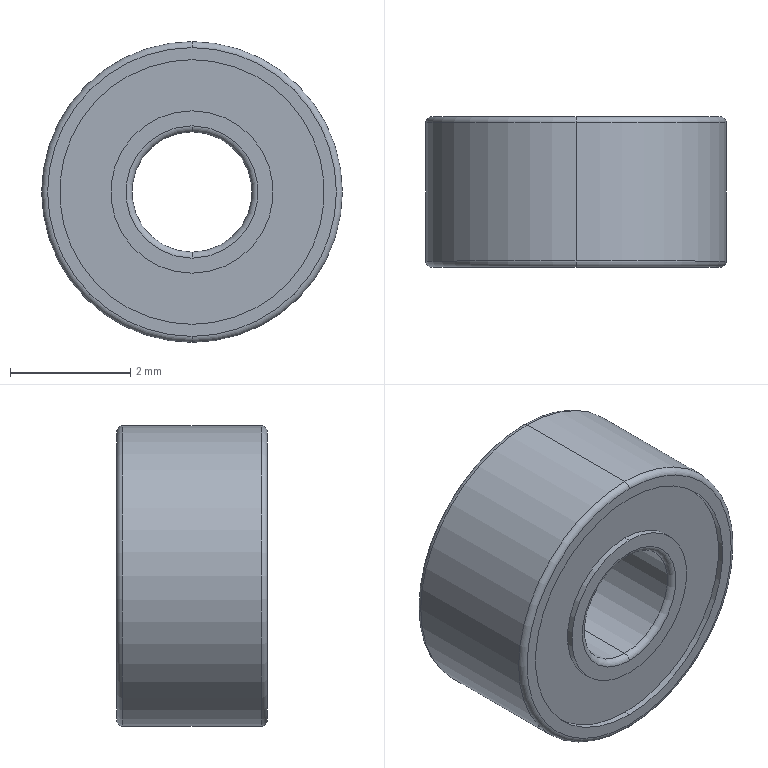Part | SolidWorks | features ICE 2, Extrusion 1, Fillet 1 | 1 solid | 26 faces | box 5 x 2.5 x 5 mm | volume 39.243 mm3 | cylinder 12 | torus 8 | plane 6 | commonest cylinder face diameters 2.7 x4 4.4 x4 2 x2 5 x2
STEP:
#1=CARTESIAN_POINT('',(0.,2.4,-2.5));
#2=VERTEX_POINT('',#1);
#3=CARTESIAN_POINT('',(0.,2.4,2.5));
#4=VERTEX_POINT('',#3);
#5=CARTESIAN_POINT('',(0.,2.4,0.));
#6=DIRECTION('',(0.,-1.,0.));
#7=DIRECTION('',(0.,0.,1.));
#8=AXIS2_PLACEMENT_3D('',#5,#6,#7);
#9=CIRCLE('',#8,2.5);
#10=EDGE_CURVE('',#2,#4,#9,.T.);
#11=ORIENTED_EDGE('',*,*,#10,.F.);
#12=CARTESIAN_POINT('',(0.,2.5,-2.4));
#13=VERTEX_POINT('',#12);
#14=CARTESIAN_POINT('',(0.,2.4,-2.4));
#15=DIRECTION('',(1.,0.,0.));
#16=DIRECTION('',(0.,0.,-1.));
#17=AXIS2_PLACEMENT_3D('',#14,#15,#16);
#18=CIRCLE('',#17,0.1);
#19=EDGE_CURVE('',#2,#13,#18,.T.);
#20=ORIENTED_EDGE('',*,*,#19,.T.);
#21=CARTESIAN_POINT('',(0.,2.5,2.4));
#22=VERTEX_POINT('',#21);
#23=CARTESIAN_POINT('',(0.,2.5,0.));
#24=DIRECTION('',(0.,1.,0.));
#25=DIRECTION('',(0.,0.,1.));
#26=AXIS2_PLACEMENT_3D('',#23,#24,#25);
#27=CIRCLE('',#26,2.4);
#28=EDGE_CURVE('',#22,#13,#27,.T.);
#29=ORIENTED_EDGE('',*,*,#28,.F.);
#30=CARTESIAN_POINT('',(0.,2.4,2.4));
#31=DIRECTION('',(-1.,0.,0.));
#32=DIRECTION('',(0.,0.,1.));
#33=AXIS2_PLACEMENT_3D('',#30,#31,#32);
#34=CIRCLE('',#33,0.1);
#35=EDGE_CURVE('',#4,#22,#34,.T.);
#36=ORIENTED_EDGE('',*,*,#35,.F.);
#37=EDGE_LOOP('',(#11,#20,#29,#36));
#38=FACE_OUTER_BOUND('',#37,.T.);
#39=CARTESIAN_POINT('',(0.,2.4,0.));
#40=DIRECTION('',(0.,1.,0.));
#41=DIRECTION('',(0.,0.,1.));
#42=AXIS2_PLACEMENT_3D('',#39,#40,#41);
#43=TOROIDAL_SURFACE('',#42,2.4,0.1);
#44=ADVANCED_FACE('',(#38),#43,.T.);
#45=CARTESIAN_POINT('',(0.,0.,-2.4));
#46=VERTEX_POINT('',#45);
#47=CARTESIAN_POINT('',(0.,0.,2.4));
#48=VERTEX_POINT('',#47);
#49=CARTESIAN_POINT('',(0.,0.,0.));
#50=DIRECTION('',(0.,-1.,0.));
#51=DIRECTION('',(0.,0.,1.));
#52=AXIS2_PLACEMENT_3D('',#49,#50,#51);
#53=CIRCLE('',#52,2.4);
#54=EDGE_CURVE('',#46,#48,#53,.T.);
#55=ORIENTED_EDGE('',*,*,#54,.F.);
#56=CARTESIAN_POINT('',(0.,0.1,-2.5));
#57=VERTEX_POINT('',#56);
#58=CARTESIAN_POINT('',(0.,0.1,-2.4));
#59=DIRECTION('',(1.,0.,0.));
#60=DIRECTION('',(0.,0.,-1.));
#61=AXIS2_PLACEMENT_3D('',#58,#59,#60);
#62=CIRCLE('',#61,0.1);
#63=EDGE_CURVE('',#46,#57,#62,.T.);
#64=ORIENTED_EDGE('',*,*,#63,.T.);
#65=CARTESIAN_POINT('',(0.,0.1,2.5));
#66=VERTEX_POINT('',#65);
#67=CARTESIAN_POINT('',(0.,0.1,0.));
#68=DIRECTION('',(0.,1.,0.));
#69=DIRECTION('',(0.,0.,1.));
#70=AXIS2_PLACEMENT_3D('',#67,#68,#69);
#71=CIRCLE('',#70,2.5);
#72=EDGE_CURVE('',#66,#57,#71,.T.);
#73=ORIENTED_EDGE('',*,*,#72,.F.);
#74=CARTESIAN_POINT('',(0.,0.1,2.4));
#75=DIRECTION('',(-1.,0.,0.));
#76=DIRECTION('',(0.,0.,1.));
#77=AXIS2_PLACEMENT_3D('',#74,#75,#76);
#78=CIRCLE('',#77,0.1);
#79=EDGE_CURVE('',#48,#66,#78,.T.);
#80=ORIENTED_EDGE('',*,*,#79,.F.);
#81=EDGE_LOOP('',(#55,#64,#73,#80));
#82=FACE_OUTER_BOUND('',#81,.T.);
#83=CARTESIAN_POINT('',(0.,0.1,0.));
#84=DIRECTION('',(0.,1.,0.));
#85=DIRECTION('',(0.,0.,1.));
#86=AXIS2_PLACEMENT_3D('',#83,#84,#85);
#87=TOROIDAL_SURFACE('',#86,2.4,0.1);
#88=ADVANCED_FACE('',(#82),#87,.T.);
#89=CARTESIAN_POINT('',(0.,2.5,-1.1));
#90=VERTEX_POINT('',#89);
#91=CARTESIAN_POINT('',(0.,2.5,1.1));
#92=VERTEX_POINT('',#91);
#93=CARTESIAN_POINT('',(0.,2.5,0.));
#94=DIRECTION('',(0.,-1.,0.));
#95=DIRECTION('',(0.,0.,1.));
#96=AXIS2_PLACEMENT_3D('',#93,#94,#95);
#97=CIRCLE('',#96,1.1);
#98=EDGE_CURVE('',#90,#92,#97,.T.);
#99=ORIENTED_EDGE('',*,*,#98,.F.);
#100=CARTESIAN_POINT('',(0.,2.4,-1.));
#101=VERTEX_POINT('',#100);
#102=CARTESIAN_POINT('',(0.,2.4,-1.1));
#103=DIRECTION('',(1.,0.,0.));
#104=DIRECTION('',(0.,0.,-1.));
#105=AXIS2_PLACEMENT_3D('',#102,#103,#104);
#106=CIRCLE('',#105,0.1);
#107=EDGE_CURVE('',#90,#101,#106,.T.);
#108=ORIENTED_EDGE('',*,*,#107,.T.);
#109=CARTESIAN_POINT('',(0.,2.4,1.));
#110=VERTEX_POINT('',#109);
#111=CARTESIAN_POINT('',(0.,2.4,0.));
#112=DIRECTION('',(0.,1.,0.));
#113=DIRECTION('',(0.,0.,1.));
#114=AXIS2_PLACEMENT_3D('',#111,#112,#113);
#115=CIRCLE('',#114,1.);
#116=EDGE_CURVE('',#110,#101,#115,.T.);
#117=ORIENTED_EDGE('',*,*,#116,.F.);
#118=CARTESIAN_POINT('',(0.,2.4,1.1));
#119=DIRECTION('',(-1.,0.,0.));
#120=DIRECTION('',(0.,0.,1.));
#121=AXIS2_PLACEMENT_3D('',#118,#119,#120);
#122=CIRCLE('',#121,0.1);
#123=EDGE_CURVE('',#92,#110,#122,.T.);
#124=ORIENTED_EDGE('',*,*,#123,.F.);
#125=EDGE_LOOP('',(#99,#108,#117,#124));
#126=FACE_OUTER_BOUND('',#125,.T.);
#127=CARTESIAN_POINT('',(0.,2.4,0.));
#128=DIRECTION('',(0.,1.,0.));
#129=DIRECTION('',(0.,0.,1.));
#130=AXIS2_PLACEMENT_3D('',#127,#128,#129);
#131=TOROIDAL_SURFACE('',#130,1.1,0.1);
#132=ADVANCED_FACE('',(#126),#131,.T.);
#133=CARTESIAN_POINT('',(0.,0.1,-1.));
#134=VERTEX_POINT('',#133);
#135=CARTESIAN_POINT('',(0.,0.1,1.));
#136=VERTEX_POINT('',#135);
#137=CARTESIAN_POINT('',(0.,0.1,0.));
#138=DIRECTION('',(0.,-1.,0.));
#139=DIRECTION('',(0.,0.,1.));
#140=AXIS2_PLACEMENT_3D('',#137,#138,#139);
#141=CIRCLE('',#140,1.);
#142=EDGE_CURVE('',#134,#136,#141,.T.);
#143=ORIENTED_EDGE('',*,*,#142,.F.);
#144=CARTESIAN_POINT('',(0.,0.,-1.1));
#145=VERTEX_POINT('',#144);
#146=CARTESIAN_POINT('',(0.,0.1,-1.1));
#147=DIRECTION('',(1.,0.,0.));
#148=DIRECTION('',(0.,0.,-1.));
#149=AXIS2_PLACEMENT_3D('',#146,#147,#148);
#150=CIRCLE('',#149,0.1);
#151=EDGE_CURVE('',#134,#145,#150,.T.);
#152=ORIENTED_EDGE('',*,*,#151,.T.);
#153=CARTESIAN_POINT('',(0.,0.,1.1));
#154=VERTEX_POINT('',#153);
#155=CARTESIAN_POINT('',(0.,0.,0.));
#156=DIRECTION('',(0.,1.,0.));
#157=DIRECTION('',(0.,0.,1.));
#158=AXIS2_PLACEMENT_3D('',#155,#156,#157);
#159=CIRCLE('',#158,1.1);
#160=EDGE_CURVE('',#154,#145,#159,.T.);
#161=ORIENTED_EDGE('',*,*,#160,.F.);
#162=CARTESIAN_POINT('',(0.,0.1,1.1));
#163=DIRECTION('',(-1.,0.,0.));
#164=DIRECTION('',(0.,0.,1.));
#165=AXIS2_PLACEMENT_3D('',#162,#163,#164);
#166=CIRCLE('',#165,0.1);
#167=EDGE_CURVE('',#136,#154,#166,.T.);
#168=ORIENTED_EDGE('',*,*,#167,.F.);
#169=EDGE_LOOP('',(#143,#152,#161,#168));
#170=FACE_OUTER_BOUND('',#169,.T.);
#171=CARTESIAN_POINT('',(0.,0.1,0.));
#172=DIRECTION('',(0.,1.,0.));
#173=DIRECTION('',(0.,0.,1.));
#174=AXIS2_PLACEMENT_3D('',#171,#172,#173);
#175=TOROIDAL_SURFACE('',#174,1.1,0.1);
#176=ADVANCED_FACE('',(#170),#175,.T.);
#177=CARTESIAN_POINT('',(0.,0.1,-1.35));
#178=VERTEX_POINT('',#177);
#179=CARTESIAN_POINT('',(0.,0.1,1.35));
#180=VERTEX_POINT('',#179);
#181=CARTESIAN_POINT('',(0.,0.1,0.));
#182=DIRECTION('',(0.,-1.,0.));
#183=DIRECTION('',(0.,0.,-1.));
#184=AXIS2_PLACEMENT_3D('',#181,#182,#183);
#185=CIRCLE('',#184,1.35);
#186=EDGE_CURVE('',#178,#180,#185,.T.);
#187=ORIENTED_EDGE('',*,*,#186,.T.);
#188=CARTESIAN_POINT('',(0.,0.,1.35));
#189=VERTEX_POINT('',#188);
#190=CARTESIAN_POINT('',(0.,0.1,1.35));
#191=DIRECTION('',(0.,-1.,0.));
#192=VECTOR('',#191,1000.);
#193=LINE('',#190,#192);
#194=EDGE_CURVE('',#180,#189,#193,.T.);
#195=ORIENTED_EDGE('',*,*,#194,.T.);
#196=CARTESIAN_POINT('',(0.,0.,-1.35));
#197=VERTEX_POINT('',#196);
#198=CARTESIAN_POINT('',(0.,0.,0.));
#199=DIRECTION('',(0.,-1.,0.));
#200=DIRECTION('',(0.,0.,-1.));
#201=AXIS2_PLACEMENT_3D('',#198,#199,#200);
#202=CIRCLE('',#201,1.35);
#203=EDGE_CURVE('',#197,#189,#202,.T.);
#204=ORIENTED_EDGE('',*,*,#203,.F.);
#205=CARTESIAN_POINT('',(0.,0.1,-1.35));
#206=DIRECTION('',(0.,-1.,0.));
#207=VECTOR('',#206,1000.);
#208=LINE('',#205,#207);
#209=EDGE_CURVE('',#178,#197,#208,.T.);
#210=ORIENTED_EDGE('',*,*,#209,.F.);
#211=EDGE_LOOP('',(#187,#195,#204,#210));
#212=FACE_OUTER_BOUND('',#211,.T.);
#213=CARTESIAN_POINT('',(0.,0.1,0.));
#214=DIRECTION('',(0.,-1.,0.));
#215=DIRECTION('',(0.,0.,-1.));
#216=AXIS2_PLACEMENT_3D('',#213,#214,#215);
#217=CYLINDRICAL_SURFACE('',#216,1.35);
#218=ADVANCED_FACE('',(#212),#217,.T.);
#219=CARTESIAN_POINT('',(0.,0.1,2.2));
#220=VERTEX_POINT('',#219);
#221=CARTESIAN_POINT('',(0.,0.1,-2.2));
#222=VERTEX_POINT('',#221);
#223=CARTESIAN_POINT('',(0.,0.1,0.));
#224=DIRECTION('',(0.,-1.,0.));
#225=DIRECTION('',(0.,0.,-1.));
#226=AXIS2_PLACEMENT_3D('',#223,#224,#225);
#227=CIRCLE('',#226,2.2);
#228=EDGE_CURVE('',#220,#222,#227,.T.);
#229=ORIENTED_EDGE('',*,*,#228,.F.);
#230=CARTESIAN_POINT('',(0.,0.,2.2));
#231=VERTEX_POINT('',#230);
#232=CARTESIAN_POINT('',(0.,0.1,2.2));
#233=DIRECTION('',(0.,-1.,0.));
#234=VECTOR('',#233,1000.);
#235=LINE('',#232,#234);
#236=EDGE_CURVE('',#220,#231,#235,.T.);
#237=ORIENTED_EDGE('',*,*,#236,.T.);
#238=CARTESIAN_POINT('',(0.,0.,-2.2));
#239=VERTEX_POINT('',#238);
#240=CARTESIAN_POINT('',(0.,0.,0.));
#241=DIRECTION('',(0.,-1.,0.));
#242=DIRECTION('',(0.,0.,-1.));
#243=AXIS2_PLACEMENT_3D('',#240,#241,#242);
#244=CIRCLE('',#243,2.2);
#245=EDGE_CURVE('',#231,#239,#244,.T.);
#246=ORIENTED_EDGE('',*,*,#245,.T.);
#247=CARTESIAN_POINT('',(0.,0.1,-2.2));
#248=DIRECTION('',(0.,-1.,0.));
#249=VECTOR('',#248,1000.);
#250=LINE('',#247,#249);
#251=EDGE_CURVE('',#222,#239,#250,.T.);
#252=ORIENTED_EDGE('',*,*,#251,.F.);
#253=EDGE_LOOP('',(#229,#237,#246,#252));
#254=FACE_OUTER_BOUND('',#253,.T.);
#255=CARTESIAN_POINT('',(0.,0.1,0.));
#256=DIRECTION('',(0.,-1.,0.));
#257=DIRECTION('',(0.,0.,-1.));
#258=AXIS2_PLACEMENT_3D('',#255,#256,#257);
#259=CYLINDRICAL_SURFACE('',#258,2.2);
#260=ADVANCED_FACE('',(#254),#259,.F.);
#261=CARTESIAN_POINT('',(0.,2.4,1.35));
#262=VERTEX_POINT('',#261);
#263=CARTESIAN_POINT('',(0.,2.4,-1.35));
#264=VERTEX_POINT('',#263);
#265=CARTESIAN_POINT('',(0.,2.4,0.));
#266=DIRECTION('',(0.,1.,0.));
#267=DIRECTION('',(0.,0.,1.));
#268=AXIS2_PLACEMENT_3D('',#265,#266,#267);
#269=CIRCLE('',#268,1.35);
#270=EDGE_CURVE('',#262,#264,#269,.T.);
#271=ORIENTED_EDGE('',*,*,#270,.T.);
#272=CARTESIAN_POINT('',(0.,2.5,-1.35));
#273=VERTEX_POINT('',#272);
#274=CARTESIAN_POINT('',(0.,2.4,-1.35));
#275=DIRECTION('',(0.,1.,0.));
#276=VECTOR('',#275,1000.);
#277=LINE('',#274,#276);
#278=EDGE_CURVE('',#264,#273,#277,.T.);
#279=ORIENTED_EDGE('',*,*,#278,.T.);
#280=CARTESIAN_POINT('',(0.,2.5,1.35));
#281=VERTEX_POINT('',#280);
#282=CARTESIAN_POINT('',(0.,2.5,0.));
#283=DIRECTION('',(0.,1.,0.));
#284=DIRECTION('',(0.,0.,1.));
#285=AXIS2_PLACEMENT_3D('',#282,#283,#284);
#286=CIRCLE('',#285,1.35);
#287=EDGE_CURVE('',#281,#273,#286,.T.);
#288=ORIENTED_EDGE('',*,*,#287,.F.);
#289=CARTESIAN_POINT('',(0.,2.4,1.35));
#290=DIRECTION('',(0.,1.,0.));
#291=VECTOR('',#290,1000.);
#292=LINE('',#289,#291);
#293=EDGE_CURVE('',#262,#281,#292,.T.);
#294=ORIENTED_EDGE('',*,*,#293,.F.);
#295=EDGE_LOOP('',(#271,#279,#288,#294));
#296=FACE_OUTER_BOUND('',#295,.T.);
#297=CARTESIAN_POINT('',(0.,2.4,0.));
#298=DIRECTION('',(0.,1.,0.));
#299=DIRECTION('',(0.,0.,1.));
#300=AXIS2_PLACEMENT_3D('',#297,#298,#299);
#301=CYLINDRICAL_SURFACE('',#300,1.35);
#302=ADVANCED_FACE('',(#296),#301,.T.);
#303=CARTESIAN_POINT('',(0.,2.4,-2.2));
#304=VERTEX_POINT('',#303);
#305=CARTESIAN_POINT('',(0.,2.4,2.2));
#306=VERTEX_POINT('',#305);
#307=CARTESIAN_POINT('',(0.,2.4,0.));
#308=DIRECTION('',(0.,1.,0.));
#309=DIRECTION('',(0.,0.,1.));
#310=AXIS2_PLACEMENT_3D('',#307,#308,#309);
#311=CIRCLE('',#310,2.2);
#312=EDGE_CURVE('',#304,#306,#311,.T.);
#313=ORIENTED_EDGE('',*,*,#312,.F.);
#314=CARTESIAN_POINT('',(0.,2.5,-2.2));
#315=VERTEX_POINT('',#314);
#316=CARTESIAN_POINT('',(0.,2.4,-2.2));
#317=DIRECTION('',(0.,1.,0.));
#318=VECTOR('',#317,1000.);
#319=LINE('',#316,#318);
#320=EDGE_CURVE('',#304,#315,#319,.T.);
#321=ORIENTED_EDGE('',*,*,#320,.T.);
#322=CARTESIAN_POINT('',(0.,2.5,2.2));
#323=VERTEX_POINT('',#322);
#324=CARTESIAN_POINT('',(0.,2.5,0.));
#325=DIRECTION('',(0.,1.,0.));
#326=DIRECTION('',(0.,0.,1.));
#327=AXIS2_PLACEMENT_3D('',#324,#325,#326);
#328=CIRCLE('',#327,2.2);
#329=EDGE_CURVE('',#315,#323,#328,.T.);
#330=ORIENTED_EDGE('',*,*,#329,.T.);
#331=CARTESIAN_POINT('',(0.,2.4,2.2));
#332=DIRECTION('',(0.,1.,0.));
#333=VECTOR('',#332,1000.);
#334=LINE('',#331,#333);
#335=EDGE_CURVE('',#306,#323,#334,.T.);
#336=ORIENTED_EDGE('',*,*,#335,.F.);
#337=EDGE_LOOP('',(#313,#321,#330,#336));
#338=FACE_OUTER_BOUND('',#337,.T.);
#339=CARTESIAN_POINT('',(0.,2.4,0.));
#340=DIRECTION('',(0.,1.,0.));
#341=DIRECTION('',(0.,0.,1.));
#342=AXIS2_PLACEMENT_3D('',#339,#340,#341);
#343=CYLINDRICAL_SURFACE('',#342,2.2);
#344=ADVANCED_FACE('',(#338),#343,.F.);
#345=CARTESIAN_POINT('',(0.,2.4,0.));
#346=DIRECTION('',(0.,1.,0.));
#347=DIRECTION('',(0.,0.,1.));
#348=AXIS2_PLACEMENT_3D('',#345,#346,#347);
#349=CIRCLE('',#348,1.);
#350=EDGE_CURVE('',#101,#110,#349,.T.);
#351=ORIENTED_EDGE('',*,*,#350,.T.);
#352=CARTESIAN_POINT('',(0.,2.5,1.));
#353=DIRECTION('',(0.,-1.,0.));
#354=VECTOR('',#353,1000.);
#355=LINE('',#352,#354);
#356=EDGE_CURVE('',#110,#136,#355,.T.);
#357=ORIENTED_EDGE('',*,*,#356,.T.);
#358=CARTESIAN_POINT('',(0.,0.1,0.));
#359=DIRECTION('',(0.,-1.,0.));
#360=DIRECTION('',(0.,0.,1.));
#361=AXIS2_PLACEMENT_3D('',#358,#359,#360);
#362=CIRCLE('',#361,1.);
#363=EDGE_CURVE('',#136,#134,#362,.T.);
#364=ORIENTED_EDGE('',*,*,#363,.T.);
#365=CARTESIAN_POINT('',(0.,2.5,-1.));
#366=DIRECTION('',(0.,-1.,0.));
#367=VECTOR('',#366,1000.);
#368=LINE('',#365,#367);
#369=EDGE_CURVE('',#101,#134,#368,.T.);
#370=ORIENTED_EDGE('',*,*,#369,.F.);
#371=EDGE_LOOP('',(#351,#357,#364,#370));
#372=FACE_OUTER_BOUND('',#371,.T.);
#373=CARTESIAN_POINT('',(0.,2.5,0.));
#374=DIRECTION('',(0.,-1.,0.));
#375=DIRECTION('',(0.,0.,-1.));
#376=AXIS2_PLACEMENT_3D('',#373,#374,#375);
#377=CYLINDRICAL_SURFACE('',#376,1.);
#378=ADVANCED_FACE('',(#372),#377,.F.);
#379=ORIENTED_EDGE('',*,*,#10,.T.);
#380=CARTESIAN_POINT('',(0.,2.5,2.5));
#381=DIRECTION('',(0.,-1.,0.));
#382=VECTOR('',#381,1000.);
#383=LINE('',#380,#382);
#384=EDGE_CURVE('',#4,#66,#383,.T.);
#385=ORIENTED_EDGE('',*,*,#384,.T.);
#386=ORIENTED_EDGE('',*,*,#72,.T.);
#387=CARTESIAN_POINT('',(0.,2.5,-2.5));
#388=DIRECTION('',(0.,-1.,0.));
#389=VECTOR('',#388,1000.);
#390=LINE('',#387,#389);
#391=EDGE_CURVE('',#2,#57,#390,.T.);
#392=ORIENTED_EDGE('',*,*,#391,.F.);
#393=EDGE_LOOP('',(#379,#385,#386,#392));
#394=FACE_OUTER_BOUND('',#393,.T.);
#395=CARTESIAN_POINT('',(0.,2.5,0.));
#396=DIRECTION('',(0.,-1.,0.));
#397=DIRECTION('',(0.,0.,-1.));
#398=AXIS2_PLACEMENT_3D('',#395,#396,#397);
#399=CYLINDRICAL_SURFACE('',#398,2.5);
#400=ADVANCED_FACE('',(#394),#399,.T.);
#401=ORIENTED_EDGE('',*,*,#160,.T.);
#402=CARTESIAN_POINT('',(0.,0.,0.));
#403=DIRECTION('',(0.,1.,0.));
#404=DIRECTION('',(0.,0.,1.));
#405=AXIS2_PLACEMENT_3D('',#402,#403,#404);
#406=CIRCLE('',#405,1.1);
#407=EDGE_CURVE('',#145,#154,#406,.T.);
#408=ORIENTED_EDGE('',*,*,#407,.T.);
#409=EDGE_LOOP('',(#401,#408));
#410=FACE_BOUND('',#409,.T.);
#411=ORIENTED_EDGE('',*,*,#203,.T.);
#412=CARTESIAN_POINT('',(0.,0.,0.));
#413=DIRECTION('',(0.,-1.,0.));
#414=DIRECTION('',(0.,0.,-1.));
#415=AXIS2_PLACEMENT_3D('',#412,#413,#414);
#416=CIRCLE('',#415,1.35);
#417=EDGE_CURVE('',#189,#197,#416,.T.);
#418=ORIENTED_EDGE('',*,*,#417,.T.);
#419=EDGE_LOOP('',(#411,#418));
#420=FACE_OUTER_BOUND('',#419,.T.);
#421=CARTESIAN_POINT('',(0.,0.,0.));
#422=DIRECTION('',(0.,1.,0.));
#423=DIRECTION('',(0.,0.,1.));
#424=AXIS2_PLACEMENT_3D('',#421,#422,#423);
#425=PLANE('',#424);
#426=ADVANCED_FACE('',(#410,#420),#425,.F.);
#427=CARTESIAN_POINT('',(0.,2.5,0.));
#428=DIRECTION('',(0.,-1.,0.));
#429=DIRECTION('',(0.,0.,1.));
#430=AXIS2_PLACEMENT_3D('',#427,#428,#429);
#431=CIRCLE('',#430,1.1);
#432=EDGE_CURVE('',#92,#90,#431,.T.);
#433=ORIENTED_EDGE('',*,*,#432,.T.);
#434=ORIENTED_EDGE('',*,*,#98,.T.);
#435=EDGE_LOOP('',(#433,#434));
#436=FACE_BOUND('',#435,.T.);
#437=ORIENTED_EDGE('',*,*,#287,.T.);
#438=CARTESIAN_POINT('',(0.,2.5,0.));
#439=DIRECTION('',(0.,1.,0.));
#440=DIRECTION('',(0.,0.,1.));
#441=AXIS2_PLACEMENT_3D('',#438,#439,#440);
#442=CIRCLE('',#441,1.35);
#443=EDGE_CURVE('',#273,#281,#442,.T.);
#444=ORIENTED_EDGE('',*,*,#443,.T.);
#445=EDGE_LOOP('',(#437,#444));
#446=FACE_OUTER_BOUND('',#445,.T.);
#447=CARTESIAN_POINT('',(0.,2.5,0.));
#448=DIRECTION('',(0.,1.,0.));
#449=DIRECTION('',(0.,0.,1.));
#450=AXIS2_PLACEMENT_3D('',#447,#448,#449);
#451=PLANE('',#450);
#452=ADVANCED_FACE('',(#436,#446),#451,.T.);
#453=ORIENTED_EDGE('',*,*,#28,.T.);
#454=CARTESIAN_POINT('',(0.,2.5,0.));
#455=DIRECTION('',(0.,1.,0.));
#456=DIRECTION('',(0.,0.,1.));
#457=AXIS2_PLACEMENT_3D('',#454,#455,#456);
#458=CIRCLE('',#457,2.4);
#459=EDGE_CURVE('',#13,#22,#458,.T.);
#460=ORIENTED_EDGE('',*,*,#459,.T.);
#461=EDGE_LOOP('',(#453,#460));
#462=FACE_OUTER_BOUND('',#461,.T.);
#463=CARTESIAN_POINT('',(0.,2.5,0.));
#464=DIRECTION('',(0.,1.,0.));
#465=DIRECTION('',(0.,0.,1.));
#466=AXIS2_PLACEMENT_3D('',#463,#464,#465);
#467=CIRCLE('',#466,2.2);
#468=EDGE_CURVE('',#323,#315,#467,.T.);
#469=ORIENTED_EDGE('',*,*,#468,.F.);
#470=ORIENTED_EDGE('',*,*,#329,.F.);
#471=EDGE_LOOP('',(#469,#470));
#472=FACE_BOUND('',#471,.T.);
#473=CARTESIAN_POINT('',(0.,2.5,0.));
#474=DIRECTION('',(0.,1.,0.));
#475=DIRECTION('',(0.,0.,1.));
#476=AXIS2_PLACEMENT_3D('',#473,#474,#475);
#477=PLANE('',#476);
#478=ADVANCED_FACE('',(#462,#472),#477,.T.);
#479=CARTESIAN_POINT('',(0.,0.,0.));
#480=DIRECTION('',(0.,-1.,0.));
#481=DIRECTION('',(0.,0.,1.));
#482=AXIS2_PLACEMENT_3D('',#479,#480,#481);
#483=CIRCLE('',#482,2.4);
#484=EDGE_CURVE('',#48,#46,#483,.T.);
#485=ORIENTED_EDGE('',*,*,#484,.T.);
#486=ORIENTED_EDGE('',*,*,#54,.T.);
#487=EDGE_LOOP('',(#485,#486));
#488=FACE_OUTER_BOUND('',#487,.T.);
#489=CARTESIAN_POINT('',(0.,0.,0.));
#490=DIRECTION('',(0.,-1.,0.));
#491=DIRECTION('',(0.,0.,-1.));
#492=AXIS2_PLACEMENT_3D('',#489,#490,#491);
#493=CIRCLE('',#492,2.2);
#494=EDGE_CURVE('',#239,#231,#493,.T.);
#495=ORIENTED_EDGE('',*,*,#494,.F.);
#496=ORIENTED_EDGE('',*,*,#245,.F.);
#497=EDGE_LOOP('',(#495,#496));
#498=FACE_BOUND('',#497,.T.);
#499=CARTESIAN_POINT('',(0.,0.,0.));
#500=DIRECTION('',(0.,1.,0.));
#501=DIRECTION('',(0.,0.,1.));
#502=AXIS2_PLACEMENT_3D('',#499,#500,#501);
#503=PLANE('',#502);
#504=ADVANCED_FACE('',(#488,#498),#503,.F.);
#505=ORIENTED_EDGE('',*,*,#384,.F.);
#506=CARTESIAN_POINT('',(0.,2.4,0.));
#507=DIRECTION('',(0.,-1.,0.));
#508=DIRECTION('',(0.,0.,1.));
#509=AXIS2_PLACEMENT_3D('',#506,#507,#508);
#510=CIRCLE('',#509,2.5);
#511=EDGE_CURVE('',#4,#2,#510,.T.);
#512=ORIENTED_EDGE('',*,*,#511,.T.);
#513=ORIENTED_EDGE('',*,*,#391,.T.);
#514=CARTESIAN_POINT('',(0.,0.1,0.));
#515=DIRECTION('',(0.,1.,0.));
#516=DIRECTION('',(0.,0.,1.));
#517=AXIS2_PLACEMENT_3D('',#514,#515,#516);
#518=CIRCLE('',#517,2.5);
#519=EDGE_CURVE('',#57,#66,#518,.T.);
#520=ORIENTED_EDGE('',*,*,#519,.T.);
#521=EDGE_LOOP('',(#505,#512,#513,#520));
#522=FACE_OUTER_BOUND('',#521,.T.);
#523=CARTESIAN_POINT('',(0.,2.5,0.));
#524=DIRECTION('',(0.,-1.,0.));
#525=DIRECTION('',(0.,0.,-1.));
#526=AXIS2_PLACEMENT_3D('',#523,#524,#525);
#527=CYLINDRICAL_SURFACE('',#526,2.5);
#528=ADVANCED_FACE('',(#522),#527,.T.);
#529=ORIENTED_EDGE('',*,*,#356,.F.);
#530=ORIENTED_EDGE('',*,*,#116,.T.);
#531=ORIENTED_EDGE('',*,*,#369,.T.);
#532=ORIENTED_EDGE('',*,*,#142,.T.);
#533=EDGE_LOOP('',(#529,#530,#531,#532));
#534=FACE_OUTER_BOUND('',#533,.T.);
#535=CARTESIAN_POINT('',(0.,2.5,0.));
#536=DIRECTION('',(0.,-1.,0.));
#537=DIRECTION('',(0.,0.,-1.));
#538=AXIS2_PLACEMENT_3D('',#535,#536,#537);
#539=CYLINDRICAL_SURFACE('',#538,1.);
#540=ADVANCED_FACE('',(#534),#539,.F.);
#541=ORIENTED_EDGE('',*,*,#320,.F.);
#542=CARTESIAN_POINT('',(0.,2.4,0.));
#543=DIRECTION('',(0.,1.,0.));
#544=DIRECTION('',(0.,0.,1.));
#545=AXIS2_PLACEMENT_3D('',#542,#543,#544);
#546=CIRCLE('',#545,2.2);
#547=EDGE_CURVE('',#306,#304,#546,.T.);
#548=ORIENTED_EDGE('',*,*,#547,.F.);
#549=ORIENTED_EDGE('',*,*,#335,.T.);
#550=ORIENTED_EDGE('',*,*,#468,.T.);
#551=EDGE_LOOP('',(#541,#548,#549,#550));
#552=FACE_OUTER_BOUND('',#551,.T.);
#553=CARTESIAN_POINT('',(0.,2.4,0.));
#554=DIRECTION('',(0.,1.,0.));
#555=DIRECTION('',(0.,0.,1.));
#556=AXIS2_PLACEMENT_3D('',#553,#554,#555);
#557=CYLINDRICAL_SURFACE('',#556,2.2);
#558=ADVANCED_FACE('',(#552),#557,.F.);
#559=ORIENTED_EDGE('',*,*,#270,.F.);
#560=CARTESIAN_POINT('',(0.,2.4,0.));
#561=DIRECTION('',(0.,1.,0.));
#562=DIRECTION('',(0.,0.,1.));
#563=AXIS2_PLACEMENT_3D('',#560,#561,#562);
#564=CIRCLE('',#563,1.35);
#565=EDGE_CURVE('',#264,#262,#564,.T.);
#566=ORIENTED_EDGE('',*,*,#565,.F.);
#567=EDGE_LOOP('',(#559,#566));
#568=FACE_BOUND('',#567,.T.);
#569=ORIENTED_EDGE('',*,*,#547,.T.);
#570=ORIENTED_EDGE('',*,*,#312,.T.);
#571=EDGE_LOOP('',(#569,#570));
#572=FACE_OUTER_BOUND('',#571,.T.);
#573=CARTESIAN_POINT('',(0.,2.4,0.));
#574=DIRECTION('',(0.,1.,0.));
#575=DIRECTION('',(0.,0.,1.));
#576=AXIS2_PLACEMENT_3D('',#573,#574,#575);
#577=PLANE('',#576);
#578=ADVANCED_FACE('',(#568,#572),#577,.T.);
#579=ORIENTED_EDGE('',*,*,#278,.F.);
#580=ORIENTED_EDGE('',*,*,#565,.T.);
#581=ORIENTED_EDGE('',*,*,#293,.T.);
#582=ORIENTED_EDGE('',*,*,#443,.F.);
#583=EDGE_LOOP('',(#579,#580,#581,#582));
#584=FACE_OUTER_BOUND('',#583,.T.);
#585=CARTESIAN_POINT('',(0.,2.4,0.));
#586=DIRECTION('',(0.,1.,0.));
#587=DIRECTION('',(0.,0.,1.));
#588=AXIS2_PLACEMENT_3D('',#585,#586,#587);
#589=CYLINDRICAL_SURFACE('',#588,1.35);
#590=ADVANCED_FACE('',(#584),#589,.T.);
#591=ORIENTED_EDGE('',*,*,#236,.F.);
#592=CARTESIAN_POINT('',(0.,0.1,0.));
#593=DIRECTION('',(0.,-1.,0.));
#594=DIRECTION('',(0.,0.,-1.));
#595=AXIS2_PLACEMENT_3D('',#592,#593,#594);
#596=CIRCLE('',#595,2.2);
#597=EDGE_CURVE('',#222,#220,#596,.T.);
#598=ORIENTED_EDGE('',*,*,#597,.F.);
#599=ORIENTED_EDGE('',*,*,#251,.T.);
#600=ORIENTED_EDGE('',*,*,#494,.T.);
#601=EDGE_LOOP('',(#591,#598,#599,#600));
#602=FACE_OUTER_BOUND('',#601,.T.);
#603=CARTESIAN_POINT('',(0.,0.1,0.));
#604=DIRECTION('',(0.,-1.,0.));
#605=DIRECTION('',(0.,0.,-1.));
#606=AXIS2_PLACEMENT_3D('',#603,#604,#605);
#607=CYLINDRICAL_SURFACE('',#606,2.2);
#608=ADVANCED_FACE('',(#602),#607,.F.);
#609=ORIENTED_EDGE('',*,*,#186,.F.);
#610=CARTESIAN_POINT('',(0.,0.1,0.));
#611=DIRECTION('',(0.,-1.,0.));
#612=DIRECTION('',(0.,0.,-1.));
#613=AXIS2_PLACEMENT_3D('',#610,#611,#612);
#614=CIRCLE('',#613,1.35);
#615=EDGE_CURVE('',#180,#178,#614,.T.);
#616=ORIENTED_EDGE('',*,*,#615,.F.);
#617=EDGE_LOOP('',(#609,#616));
#618=FACE_BOUND('',#617,.T.);
#619=ORIENTED_EDGE('',*,*,#597,.T.);
#620=ORIENTED_EDGE('',*,*,#228,.T.);
#621=EDGE_LOOP('',(#619,#620));
#622=FACE_OUTER_BOUND('',#621,.T.);
#623=CARTESIAN_POINT('',(0.,0.1,0.));
#624=DIRECTION('',(0.,-1.,0.));
#625=DIRECTION('',(0.,0.,-1.));
#626=AXIS2_PLACEMENT_3D('',#623,#624,#625);
#627=PLANE('',#626);
#628=ADVANCED_FACE('',(#618,#622),#627,.T.);
#629=ORIENTED_EDGE('',*,*,#194,.F.);
#630=ORIENTED_EDGE('',*,*,#615,.T.);
#631=ORIENTED_EDGE('',*,*,#209,.T.);
#632=ORIENTED_EDGE('',*,*,#417,.F.);
#633=EDGE_LOOP('',(#629,#630,#631,#632));
#634=FACE_OUTER_BOUND('',#633,.T.);
#635=CARTESIAN_POINT('',(0.,0.1,0.));
#636=DIRECTION('',(0.,-1.,0.));
#637=DIRECTION('',(0.,0.,-1.));
#638=AXIS2_PLACEMENT_3D('',#635,#636,#637);
#639=CYLINDRICAL_SURFACE('',#638,1.35);
#640=ADVANCED_FACE('',(#634),#639,.T.);
#641=ORIENTED_EDGE('',*,*,#151,.F.);
#642=ORIENTED_EDGE('',*,*,#363,.F.);
#643=ORIENTED_EDGE('',*,*,#167,.T.);
#644=ORIENTED_EDGE('',*,*,#407,.F.);
#645=EDGE_LOOP('',(#641,#642,#643,#644));
#646=FACE_OUTER_BOUND('',#645,.T.);
#647=CARTESIAN_POINT('',(0.,0.1,0.));
#648=DIRECTION('',(0.,1.,0.));
#649=DIRECTION('',(0.,0.,1.));
#650=AXIS2_PLACEMENT_3D('',#647,#648,#649);
#651=TOROIDAL_SURFACE('',#650,1.1,0.1);
#652=ADVANCED_FACE('',(#646),#651,.T.);
#653=ORIENTED_EDGE('',*,*,#107,.F.);
#654=ORIENTED_EDGE('',*,*,#432,.F.);
#655=ORIENTED_EDGE('',*,*,#123,.T.);
#656=ORIENTED_EDGE('',*,*,#350,.F.);
#657=EDGE_LOOP('',(#653,#654,#655,#656));
#658=FACE_OUTER_BOUND('',#657,.T.);
#659=CARTESIAN_POINT('',(0.,2.4,0.));
#660=DIRECTION('',(0.,1.,0.));
#661=DIRECTION('',(0.,0.,1.));
#662=AXIS2_PLACEMENT_3D('',#659,#660,#661);
#663=TOROIDAL_SURFACE('',#662,1.1,0.1);
#664=ADVANCED_FACE('',(#658),#663,.T.);
#665=ORIENTED_EDGE('',*,*,#63,.F.);
#666=ORIENTED_EDGE('',*,*,#484,.F.);
#667=ORIENTED_EDGE('',*,*,#79,.T.);
#668=ORIENTED_EDGE('',*,*,#519,.F.);
#669=EDGE_LOOP('',(#665,#666,#667,#668));
#670=FACE_OUTER_BOUND('',#669,.T.);
#671=CARTESIAN_POINT('',(0.,0.1,0.));
#672=DIRECTION('',(0.,1.,0.));
#673=DIRECTION('',(0.,0.,1.));
#674=AXIS2_PLACEMENT_3D('',#671,#672,#673);
#675=TOROIDAL_SURFACE('',#674,2.4,0.1);
#676=ADVANCED_FACE('',(#670),#675,.T.);
#677=ORIENTED_EDGE('',*,*,#19,.F.);
#678=ORIENTED_EDGE('',*,*,#511,.F.);
#679=ORIENTED_EDGE('',*,*,#35,.T.);
#680=ORIENTED_EDGE('',*,*,#459,.F.);
#681=EDGE_LOOP('',(#677,#678,#679,#680));
#682=FACE_OUTER_BOUND('',#681,.T.);
#683=CARTESIAN_POINT('',(0.,2.4,0.));
#684=DIRECTION('',(0.,1.,0.));
#685=DIRECTION('',(0.,0.,1.));
#686=AXIS2_PLACEMENT_3D('',#683,#684,#685);
#687=TOROIDAL_SURFACE('',#686,2.4,0.1);
#688=ADVANCED_FACE('',(#682),#687,.T.);
#689=CLOSED_SHELL('',(#44,#88,#132,#176,#218,#260,#302,#344,#378,#400,#426,#452,#478,#504,#528,#540,#558,#578,#590,#608,#628,#640,#652,#664,#676,#688));
#690=MANIFOLD_SOLID_BREP('',#689);
#691=CARTESIAN_POINT('',(0.,0.,0.));
#692=DIRECTION('',(0.,0.,1.));
#693=DIRECTION('',(1.,0.,0.));
#694=AXIS2_PLACEMENT_3D('',#691,#692,#693);
#695=(LENGTH_UNIT()NAMED_UNIT(*)SI_UNIT(.MILLI.,.METRE.));
#696=UNCERTAINTY_MEASURE_WITH_UNIT(LENGTH_MEASURE(0.00001),#695,'','');
#697=(NAMED_UNIT(*)PLANE_ANGLE_UNIT()SI_UNIT($,.RADIAN.));
#698=(NAMED_UNIT(*)SI_UNIT($,.STERADIAN.)SOLID_ANGLE_UNIT());
#699=(GEOMETRIC_REPRESENTATION_CONTEXT(3)GLOBAL_UNCERTAINTY_ASSIGNED_CONTEXT((#696))GLOBAL_UNIT_ASSIGNED_CONTEXT((#695,#697,#698))REPRESENTATION_CONTEXT('',''));
#700=ADVANCED_BREP_SHAPE_REPRESENTATION('',(#690,#694),#699);